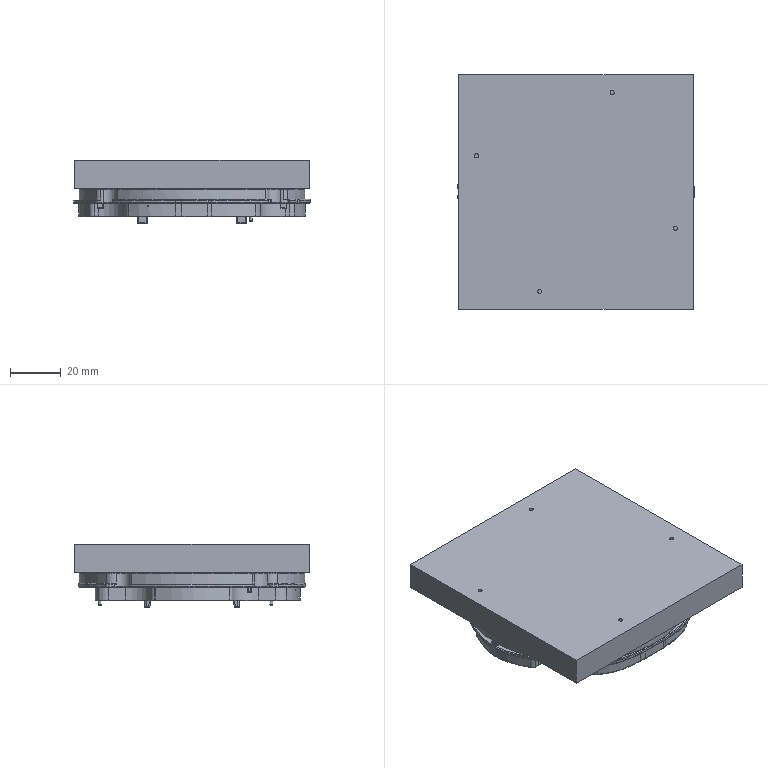NC program | NX | posted with a generic post | part box 92.935 x 92.1 x 24.829 mm
Lines 1 to 800 of 7643:
N10 G17 G21 G94 G90
(动态粗 , TOOL : D8-25-D8-60-3T-ROUGH)
N12 T10 M6
N14 G53
N16 G17 G0 G90 X-61.58 Y-2.72 S6500 M3
N18 G43 Z21. H10
N20 Z-16.5
N22 G94 G1 X-61.555 Y-2.718 Z-16.656 F3000.
N24 X-61.53 Y-2.716 Z-16.718
N26 X-61.505 Y-2.714 Z-16.763
N28 X-61.48 Y-2.712 Z-16.8
N30 X-61.455 Y-2.71 Z-16.831
N32 X-61.431 Y-2.708 Z-16.857
N34 X-61.406 Y-2.706 Z-16.88
N36 X-61.381 Y-2.704 Z-16.9
N38 X-61.356 Y-2.702 Z-16.918
N40 X-61.331 Y-2.7 Z-16.933
N42 X-61.306 Y-2.698 Z-16.947
N44 X-61.281 Y-2.696 Z-16.958
N46 X-61.256 Y-2.695 Z-16.968
N48 X-61.231 Y-2.693 Z-16.977
N50 X-61.206 Y-2.691 Z-16.984
N52 X-61.181 Y-2.689 Z-16.99
N54 X-61.156 Y-2.687 Z-16.994
N56 X-61.131 Y-2.685 Z-16.997
N58 X-61.107 Y-2.683 Z-16.999
N60 X-61.082 Y-2.681 Z-17.
N62 X-59.705 Y-2.575
N64 G3 X-59.048 Y-2.136 R0.809
N66 X-58.304 Y0.589 R7.458
N68 X-58.019 Y7.275 R66.093
N70 G1 X-57.999 Y15.352
N72 X-57.998 Y47.527
N74 G2 X-56.531 Y50.466 R4.191
N76 X-52.801 Y52.296 R8.355
N78 X-47.293 Y52.907 R28.085
N80 X-35.218 Y52.998 R429.952
N82 G1 X52.502
N84 G2 X55.445 Y51.539 R4.188
N86 X57.288 Y47.811 R8.352
N88 X57.906 Y42.305 R27.817
N90 X57.998 Y29.781 R440.504
N92 G1 X57.997 Y-47.524
N94 G2 X56.474 Y-50.512 R4.207
N96 X52.725 Y-52.312 R8.521
N98 X47.292 Y-52.907 R28.494
N100 X34.767 Y-52.998 R444.554
N102 G1 X-52.574 Y-52.996
N104 G2 X-55.546 Y-51.436 R4.252
N106 X-57.309 Y-47.741 R8.541
N108 X-57.906 Y-42.308 R28.316
N110 X-57.998 Y-29.784 R440.931
N112 G1 Y-5.349
N114 G2 X-57.574 Y-1.423 R34.883
N116 G3 X-57.04 Y7.367 R73.929
N118 X-56.999 Y17.527 R708.895
N120 G1 X-56.998 Y44.852
N122 G2 X-54.606 Y49.404 R5.85
N124 X-50.234 Y51.294 R10.717
N126 X-44.198 Y51.905 R34.632
N128 X-31.824 Y51.998 R454.909
N130 G1 X49.951 Y51.994
N132 G2 X54.419 Y49.578 R5.878
N134 X56.299 Y45.194 R10.811
N136 X56.913 Y38.933 R36.036
N138 X56.998 Y26.408 R512.708
N140 G1 X56.994 Y-44.973
N142 G2 X54.556 Y-49.44 R5.866
N144 X50.082 Y-51.323 R10.949
N146 X43.742 Y-51.919 R37.298
N148 X31.743 Y-51.998 R529.05
N150 G1 X-49.973 Y-51.994
N152 G2 X-54.479 Y-49.505 R5.891
N154 X-56.333 Y-45.038 R11.051
N156 X-56.92 Y-38.698 R37.895
N158 X-56.998 Y-26.249 R562.106
N160 G1 X-56.997 Y-7.449
N162 G2 X-56.543 Y-1.375 R62.284
N164 G3 X-56.019 Y10.497 R124.747
N166 G1 X-55.999 Y19.027
N168 X-55.998 Y42.527
N170 G2 X-52.754 Y48.527 R6.958
N172 X-47.94 Y50.343 R12.879
N174 X-41.372 Y50.916 R42.732
N176 X-28.622 Y50.997 R571.229
N178 G1 X47.528 Y50.996
N180 G2 X53.526 Y47.746 R6.968
N182 X55.341 Y42.934 R12.909
N184 X55.916 Y36.365 R42.803
N186 X55.997 Y23.541 R570.967
N188 G1 X55.996 Y-42.574
N190 G2 X52.819 Y-48.478 R6.937
N192 X48.018 Y-50.325 R12.706
N194 X41.302 Y-50.918 R42.332
N196 X28.552 Y-50.997 R585.104
N198 G1 X-47.523 Y-50.996
N200 G2 X-53.523 Y-47.754 R6.958
N202 X-55.326 Y-43.012 R12.809
N204 X-55.916 Y-36.371 R42.21
N206 X-55.997 Y-23.621 R569.284
N208 G1 X-55.996 Y-9.174
N210 G2 X-55.529 Y-1.349 R89.159
N212 G3 X-55.015 Y12.216 R166.099
N214 G1 X-54.999 Y20.452
N216 X-54.998 Y40.427
N218 G2 X-53.974 Y44.752 R8.324
N220 X-49.835 Y48.261 R8.776
N222 X-44.314 Y49.606 R18.927
N224 X-36.001 Y49.973 R85.068
N226 G1 X-26.101 Y49.997
N228 X45.377 Y49.996
N230 G2 X49.51 Y49.104 R8.517
N232 X53.139 Y45.091 R8.55
N234 X54.543 Y39.822 R17.669
N236 X54.966 Y31.662 R73.619
N238 G1 X54.997 Y20.937
N240 X54.996 Y-40.399
N242 G2 X54.094 Y-44.529 R8.451
N244 X50.067 Y-48.151 R8.576
N246 X44.642 Y-49.565 R18.027
N248 X36.556 Y-49.967 R76.51
N250 G1 X26.656 Y-49.997
N252 X-45.548 Y-49.995
N254 G2 X-50.109 Y-48.749 R8.039
N256 X-53.411 Y-44.473 R9.125
N258 X-54.661 Y-38.774 R20.599
N260 X-54.98 Y-30.083 R101.178
N262 G1 X-54.997 Y-21.008
N264 G2 X-54.956 Y-8.234 R650.637
N266 X-54.414 Y0.174 R225.645
N268 G3 X-54.007 Y14.834 R226.099
N270 G1 X-54. Y21.427
N272 X-53.997 Y38.627
N274 G2 X-53.323 Y42.594 R10.093
N276 X-49.146 Y46.885 R8.682
N278 X-43.617 Y48.48 R17.419
N280 X-36.061 Y48.945 R65.003
N282 X-24.361 Y48.997 R751.259
N284 G1 X43.614 Y48.994
N286 G2 X47.58 Y48.325 R10.167
N288 X51.868 Y44.173 R8.67
N290 X53.473 Y38.649 R17.352
N292 X53.946 Y31.018 R64.814
N294 X53.997 Y19.319 R752.456
N296 G1 X53.994 Y-38.681
N298 G2 X53.24 Y-42.78 R9.886
N300 X49.186 Y-46.86 R8.709
N302 X43.664 Y-48.47 R17.315
N304 X35.884 Y-48.948 R65.303
N306 X24.184 Y-48.996 R757.357
N308 G1 X-43.523 Y-48.995
N310 G2 X-47.427 Y-48.388 R10.486
N312 X-51.769 Y-44.358 R8.53
N314 X-53.431 Y-38.933 R16.692
N316 X-53.933 Y-31.68 R58.512
N318 X-53.997 Y-19.081 R756.083
N320 X-53.923 Y-8.124 R348.839
N322 X-53.366 Y1.045 R448.52
N324 G3 X-53.003 Y17.381 R286.219
N326 G1 X-53. Y22.327
N328 X-52.999 Y36.677
N330 G2 X-52.532 Y40.608 R13.005
N332 X-48.298 Y45.603 R8.772
N334 X-42.818 Y47.366 R16.685
N336 X-35.044 Y47.93 R57.999
N338 X-22.444 Y47.996 R751.574
N340 G1 X-12.214 Y47.997
N342 G2 X-2.428 Y48.649 R93.802
N344 X-0.938 Y48.456 R7.257
N346 G3 X0.999 Y48.473 R60.276
N348 G2 X2.359 Y48.649 R5.135
N350 X11.245 Y48.119 R116.377
N352 G3 X21.679 Y47.999 R281.98
N354 G1 X24.977 Y47.997
N356 X41.477 Y47.996
N358 G2 X45.272 Y47.626 R14.458
N360 X50.496 Y43.48 R8.662
N362 X52.329 Y38.029 R16.152
N364 X52.92 Y30.484 R54.023
N366 X52.996 Y17.809 R675.282
N368 G1 X52.994 Y-36.891
N370 G2 X52.438 Y-40.883 R12.008
N372 X48.27 Y-45.616 R8.807
N374 X42.718 Y-47.379 R16.873
N376 X34.868 Y-47.934 R59.591
N378 X22.268 Y-47.996 R759.278
N380 G1 X11.814 Y-47.997
N382 G2 X6.557 Y-48.462 R68.987
N384 X-10.972 Y-48.123 R114.357
N386 G3 X-21.625 Y-47.998 R270.066
N388 G1 X-41.374 Y-47.997
N390 G2 X-45.173 Y-47.653 R15.159
N392 X-50.487 Y-43.493 R8.652
N394 X-52.312 Y-38.122 R16.047
N396 X-52.917 Y-30.578 R52.808
N398 X-52.948 Y-9.629 R728.599
N400 X-52.409 Y0.369 R300.852
N402 G3 X-52.005 Y17.457 R297.752
N404 G1 X-52. Y22.402
N406 X-51.999 Y35.027
N408 G2 X-51.588 Y39.044 R15.182
N410 X-47.354 Y44.395 R8.967
N412 X-41.769 Y46.297 R16.488
N414 X-34.375 Y46.906 R52.937
N416 X-17.925 Y46.998 R776.352
N418 X-12.17 Y48.002 R46.605
N420 G3 X-19.006 Y46.734 R48.996
N422 G2 X-23.71 Y46.426 R32.015
N424 G3 X-35.146 Y46.267 R516.607
N426 X-42.15 Y45.534 R42.041
N428 X-47.261 Y43.465 R13.846
N430 X-50.907 Y37.704 R8.969
N432 X-51.354 Y32.556 R29.389
N434 X-51.405 Y17.729 R914.653
N436 G2 X-52.153 Y-5.249 R315.184
N438 G3 X-52.395 Y-17.47 R206.34
N440 X-52.267 Y-31.719 R423.43
N442 X-51.514 Y-38.644 R39.439
N444 X-49.463 Y-43.521 R13.03
N446 X-43.997 Y-46.903 R8.667
N448 X-38.923 Y-47.349 R29.196
N450 X-23.92 Y-47.396 R890.368
N452 G1 X-15.907 Y-47.421
N454 G3 X-10.698 Y-48.139 R66.308
N456 G2 X-18.604 Y-46.831 R55.637
N458 G3 X-23.932 Y-46.448 R37.065
N460 X-36.103 Y-46.381 R886.258
N462 G2 X-41.867 Y-46.095 R47.99
N464 X-46.751 Y-44.096 R9.428
N466 X-49.889 Y-39.361 R10.658
N468 X-51.067 Y-33.337 R24.634
N470 X-51.383 Y-23.369 R126.177
N472 X-51.305 Y-9.195 R466.749
N474 X-50.728 Y2.216 R781.354
N476 G3 X-50.404 Y19.705 R374.655
N478 G2 X-50.331 Y32.553 R530.644
N480 X-49.769 Y37.234 R21.015
N482 X-45.07 Y43.019 R9.193
N484 X-39.436 Y44.766 R17.581
N486 X-31.437 Y45.33 R61.997
N488 G3 X-22.401 Y45.493 R402.225
N490 X-20.942 Y46.075 R16.661
N492 G1 X-18.817 Y46.771
N494 G3 X-22.604 Y45.385 R31.53
N496 G2 X-25.744 Y44.909 R12.566
N498 X-33.704 Y44.648 R705.529
N500 G3 X-40.552 Y43.867 R39.499
N502 X-45.441 Y41.815 R13.41
N504 X-49.026 Y36.416 R9.392
N506 X-49.709 Y30.919 R25.341
N508 X-49.805 Y19.228 R391.929
N510 G2 X-49.981 Y6.512 R401.107
N512 G3 X-50.653 Y2.177 R33.083
N514 X-50.496 Y0.234 R12.796
N516 G2 X-50.624 Y-1.166 R2.803
N518 G3 X-50.587 Y-3.297 R17.335
N520 G2 X-50.73 Y-10.379 R211.012
N522 G3 X-50.67 Y-29.577 R444.123
N524 X-49.948 Y-36.506 R41.556
N526 X-47.926 Y-41.483 R13.371
N528 X-42.653 Y-45.017 R9.165
N530 X-37.232 Y-45.703 R24.779
N532 X-26.132 Y-45.82 R451.215
N534 G2 X-21.001 Y-46.012 R68.76
N536 G3 X-18.265 Y-46.898 R36.594
N538 G2 X-22.199 Y-45.53 R32.077
N540 G3 X-26.297 Y-44.949 R17.657
N542 X-34.934 Y-44.754 R275.021
N544 G2 X-40.608 Y-44.276 R34.269
N546 X-45.752 Y-41.66 R9.566
N548 X-48.538 Y-36.66 R11.811
N550 X-49.553 Y-30.226 R29.792
N552 X-49.787 Y-19.431 R179.128
N554 X-49.663 Y-7.748 R423.819
N556 X-50.625 Y-2.452 R36.382
N558 G3 X-49.674 Y-7.67 R35.094
N560 G2 X-49.258 Y-10.429 R10.113
N562 X-49.186 Y-19.33 R248.98
N564 G3 X-48.937 Y-30.05 R166.308
N566 X-47.909 Y-36.252 R27.806
N568 X-45.177 Y-40.933 R10.845
N570 X-40.373 Y-43.438 R10.384
N572 X-34.722 Y-44.107 R28.796
N574 G2 X-26.66 Y-44.353 R469.078
N576 X-24.143 Y-44.617 R21.733
N578 G3 X-22.172 Y-45.54 R26.904
N580 G2 X-24.917 Y-44.222 R32.855
N582 G3 X-28.254 Y-43.482 R11.563
N584 X-34.731 Y-43.094 R154.343
N586 G2 X-39.912 Y-42.322 R23.628
N588 X-46.104 Y-36.962 R9.673
N590 X-47.68 Y-31.115 R19.509
N592 X-48.139 Y-23.332 R71.778
N594 G1 X-48.209 Y-13.121
N596 G3 X-48.278 Y-11.836 R6.569
N598 G2 X-49.537 Y-8.137 R29.55
N600 G3 X-48.106 Y-12.277 R32.915
N602 G2 X-47.677 Y-15.66 R14.569
N604 X-47.499 Y-24.693 R957.139
N606 G3 X-46.872 Y-32.009 R50.54
N608 X-45.014 Y-37.292 R15.254
N610 X-39.499 Y-41.513 R9.823
N612 X-34.118 Y-42.457 R23.428
N614 G2 X-28.22 Y-42.929 R133.266
N616 X-26.525 Y-43.254 R8.785
N618 G1 X-24.718 Y-44.324
N620 G2 X-27.186 Y-42.819 R39.878
N622 G3 X-30.36 Y-41.939 R10.56
N624 G2 X-35.597 Y-41.263 R757.768
N626 X-40.36 Y-39.746 R14.148
N628 X-44.671 Y-34.763 R10.229
N630 X-46.148 Y-28.662 R21.487
N632 X-46.551 Y-21.1 R83.994
N634 G3 X-46.743 Y-15.442 R96.671
N636 X-47.494 Y-13.733 R27.048
N638 G1 X-48.181 Y-12.07
N640 G3 X-46.588 Y-15.767 R116.697
N642 G2 X-46.097 Y-18.895 R13.324
N644 G1 X-45.77 Y-25.752
N646 G3 X-44.802 Y-32.193 R31.449
N648 X-42.14 Y-37.171 R11.835
N650 X-37.218 Y-40.071 R10.973
N652 X-32.11 Y-41.072 R35.641
N654 G2 X-28.701 Y-41.755 R24.025
N656 X-27.031 Y-42.909 R28.
N658 X-29.059 Y-41.419 R22.396
N660 G3 X-31.754 Y-40.376 R9.271
N662 G2 X-36.132 Y-39.251 R75.156
N664 X-41.436 Y-35.754 R10.775
N666 X-43.922 Y-30.413 R13.767
N668 X-44.802 Y-23.957 R36.812
N670 G3 X-45.17 Y-18.68 R98.427
N672 G1 X-46.659 Y-15.585
N674 X-45.008 Y-18.983
N676 G2 X-44.404 Y-22.156 R13.593
N678 G3 X-43.708 Y-28.164 R86.126
N680 X-41.923 Y-33.553 R16.796
N682 X-36.49 Y-38.227 R10.796
N684 X-32.271 Y-39.598 R38.921
N686 G2 X-30.454 Y-40.227 R18.329
N688 G1 X-28.905 Y-41.532
N690 G2 X-30.932 Y-39.761 R34.939
N692 G3 X-33.274 Y-38.517 R11.416
N694 G2 X-37.068 Y-36.655 R24.972
N696 X-41.678 Y-30.788 R11.687
N698 X-43.019 Y-24.95 R26.219
N700 G3 X-43.438 Y-21.958 R335.773
N702 G1 X-45.081 Y-18.815
N704 G3 X-43.216 Y-22.365 R447.582
N706 G2 X-42.491 Y-25.075 R16.311
N708 G3 X-41.179 Y-30.08 R31.83
N710 X-35.498 Y-36.627 R12.158
N712 G1 X-32.491 Y-38.207
N714 X-30.792 Y-39.881
N716 G2 X-33.112 Y-37.47 R32.523
N718 G3 X-35.722 Y-35.365 R61.614
N720 G2 X-40.398 Y-28.487 R14.563
N722 X-41.206 Y-25.828 R116.518
N724 X-43.311 Y-22.161 R75.506
N726 G3 X-41.37 Y-25.584 R346.156
N728 G2 X-40.263 Y-27.536 R8.47
N730 G3 X-38.083 Y-31.671 R24.809
N732 X-34.821 Y-35.177 R19.008
N734 G2 X-33.968 Y-36.464 R91.324
N736 G1 X-32.985 Y-37.597
N738 G2 X-34.619 Y-35.498 R13.241
N740 G3 X-35.821 Y-33.292 R10.755
N742 G2 X-38.875 Y-28.029 R48.011
N744 G1 X-39.03 Y-27.866
N746 G2 X-40.705 Y-26.489 R7.646
N748 G1 X-41.06 Y-26.006
N750 X-40.705 Y-26.489
N752 G3 X-38.908 Y-27.945 R7.826
N754 G2 X-37.422 Y-29.807 R9.645
N756 X-35.461 Y-32.799 R156.161
N758 X-35.374 Y-33.303 R1.645
N760 G1 X-35.092 Y-34.434
N762 X-35.001 Y-34.639
N764 G2 X-35.425 Y-32.577 R6.115
N766 G3 X-36.662 Y-29.587 R9.097
N768 X-37.361 Y-28.611 R4.628
N770 X-37.953 Y-28.378 R1.522
N772 G1 X-38.972 Y-27.906
N774 X-37.953 Y-28.378
N776 G2 X-36.723 Y-29.1 R1.909
N778 X-35.405 Y-31.301 R6.68
N780 X-35.456 Y-32.142 R3.094
N782 G1 X-35.424 Y-32.59
N784 G2 X-35.389 Y-31.498 R3.522
N786 G3 X-35.852 Y-29.445 R3.065
N788 X-36.491 Y-28.75 R1.511
N790 G1 X-37.52 Y-28.496
N792 G3 X-36.466 Y-28.72 R4.38
N794 G2 X-35.322 Y-30.038 R2.305
N796 X-35.335 Y-30.983 R1.189
N798 G1 X-35.351 Y-31.132
N800 G2 X-35.176 Y-30.423 R5.061
N802 G3 X-35.753 Y-28.876 R1.638
N804 X-36.601 Y-28.7 R1.92
N806 G1 X-35.855 Y-28.78
N808 G2 X-35.074 Y-30.064 R1.25
N810 G1 X-35.176 Y-30.425
N812 G3 X-34.996 Y-29.647 R4.512
N814 X-35.969 Y-28.762 R0.921
N816 X-36.593 Y-28.973 R0.803
N818 G1 X-36.943 Y-29.299
N820 X-38.087 Y-30.366 Z-16.9
N822 G2 X-39.018 Y-30.522 R0.803 F15000.
N824 G1 X-39.673 Y-30.194
N826 X-40.324 Y-29.857
N828 G2 X-41.806 Y-28.867 R10.095
N830 X-42.83 Y-27.639 R4.698
N832 G1 X-44.026 Y-25.565
N834 X-45.215 Y-23.487
N836 G2 X-48.507 Y-17.159 R115.865
N838 X-51.398 Y-10.117 R71.891
N840 X-52.234 Y-7.344 R44.136
N842 X-52.741 Y-4.7 R22.374
N844 G1 X-52.958 Y-3.027
N846 G2 X-52.614 Y-2.263 R0.801
N848 G1 X-51.326 Y-1.373 Z-17. F3000.
N850 X-51.009 Y-1.157
N852 X-50.7 Y-0.931
N854 G3 X-50.468 Y-0.538 R0.814
N856 X-50.406 Y0.31 R1.534
N858 G1 X-50.625 Y1.193
N860 X-50.653 Y2.177
N862 G2 X-50.368 Y4.504 R30.875
N864 X-49.365 Y8.916 R48.271
N866 G3 X-48.895 Y14.022 R31.072
N868 X-48.781 Y26.909 R644.328
N870 G2 X-48.431 Y33.495 R52.792
N872 X-46.843 Y38.145 R11.412
N874 X-42.08 Y41.953 R10.192
N876 X-36.108 Y43.358 R21.859
N878 X-28.168 Y43.808 R109.95
N880 G3 X-25.391 Y44.004 R39.396
N882 X-24.999 Y44.204 R2.842
N884 G2 X-22.591 Y45.391 R33.125
N886 G3 X-25.524 Y43.904 R31.271
N888 G2 X-28.22 Y43.344 R9.885
N890 X-34.501 Y42.886 R755.129
N892 G3 X-40.459 Y41.769 R26.181
N894 X-45.27 Y38.67 R10.587
N896 X-47.559 Y33.677 R11.137
N898 X-48.138 Y27.488 R34.991
N900 X-48.24 Y16.873 R884.24
N902 G2 X-48.491 Y11.33 R65.646
N904 G3 X-49.467 Y8.491 R54.281
N906 G2 X-47.957 Y12.688 R50.945
N908 G3 X-47.375 Y16.666 R18.146
N910 X-47.163 Y25.885 R238.666
N912 G2 X-46.689 Y32.161 R41.673
N914 X-44.698 Y37.045 R11.146
N916 X-39.813 Y40.522 R10.861
N918 X-33.968 Y41.807 R24.231
N920 G3 X-28.421 Y42.364 R323.329
N922 X-27.564 Y42.567 R2.429
N924 G2 X-25.307 Y44.017 R24.433
N926 G3 X-27.685 Y42.479 R24.542
N928 G2 X-29.804 Y41.798 R6.558
N930 X-34.852 Y41.067 R238.638
N932 G3 X-40.171 Y39.547 R19.422
N934 X-45.552 Y33.222 R10.006
N936 X-46.451 Y27.456 R24.19
N938 X-46.689 Y18.889 R416.558
N940 G2 X-46.998 Y14.897 R37.516
N942 G1 X-47.991 Y12.581
N944 G2 X-46.498 Y15.952 R93.021
N946 G3 X-45.825 Y19.661 R14.909
N948 X-45.49 Y26.341 R291.055
N950 G2 X-44.689 Y31.897 R25.594
N952 X-39.086 Y38.472 R10.119
N954 X-33.855 Y40.055 R21.227
N956 G3 X-29.864 Y40.835 R75.673
N958 G1 X-29.606 Y40.969
N960 G2 X-27.626 Y42.522 R15.785
N962 G3 X-29.778 Y40.824 R17.362
N964 G2 X-31.96 Y39.966 R7.743
N966 G3 X-36.392 Y38.779 R77.204
N968 X-41.178 Y36.055 R12.3
N970 X-44.108 Y30.793 R11.117
N972 X-44.917 Y24.857 R30.653
N974 G2 X-45.366 Y18.74 R90.011
N976 X-45.501 Y18. R11.468
N978 G1 X-46.572 Y15.769
N980 X-44.934 Y19.18
N982 G3 X-44.207 Y22.628 R15.053
N984 G2 X-43.549 Y28.083 R105.738
N986 X-41.816 Y33.004 R13.614
N988 X-37.02 Y37.085 R11.045
N990 X-32.508 Y38.726 R38.5
N992 G3 X-31.619 Y39.096 R3.163
N994 G2 X-29.704 Y40.884 R21.086
N996 G3 X-31.778 Y38.937 R22.587
N998 G2 X-33.872 Y37.809 R9.504
N1000 G3 X-37.796 Y35.844 R25.277
N1002 X-42.323 Y29.717 R11.079
N1004 X-43.373 Y24.351 R30.532
N1006 G2 X-43.904 Y21.082 R27.325
N1008 G1 X-45.058 Y18.892
N1010 G3 X-43.242 Y22.363 R539.919
N1012 X-42.419 Y25.165 R18.609
N1014 G2 X-41.093 Y29.701 R27.337
N1016 X-36.311 Y35.175 R11.78
N1018 G1 X-33.935 Y36.559
N1020 X-32.277 Y38.443
N1022 X-31.744 Y38.971
N1024 G3 X-34.095 Y36.343 R34.059
N1026 G2 X-36.293 Y34.52 R25.762
N1028 G3 X-40.945 Y27.825 R13.716
N1030 X-41.891 Y24.704 R159.879
N1032 G1 X-43.368 Y22.093
N1034 X-41.529 Y25.345
N1036 G3 X-39.904 Y28.126 R21.532
N1038 G2 X-35.848 Y33.326 R18.403
N1040 G3 X-35.236 Y33.977 R2.888
N1042 G2 X-33.958 Y36.501 R6.809
N1044 G1 X-34.563 Y35.643
N1046 X-35.066 Y34.563
N1048 G2 X-35.8 Y32.973 R3.417
N1050 G3 X-38.567 Y29.079 R49.359
N1052 G2 X-39.474 Y27.602 R18.195
N1054 G3 X-40.952 Y26.202 R6.694
N1056 G2 X-40.053 Y27.17 R9.352
N1058 G3 X-37.072 Y29.899 R12.939
N1060 X-35.547 Y31.843 R19.81
N1062 X-35.464 Y32.223 R1.563
N1064 G1 X-35.369 Y33.411
N1066 X-35.216 Y33.991
N1068 X-35.369 Y33.411
N1070 G2 X-35.479 Y31.878 R66.65
N1072 X-36.736 Y29.643 R7.055
N1074 X-37.736 Y28.506 R8.458
N1076 G1 X-39.104 Y27.858
N1078 G2 X-37.936 Y28.402 R10.366
N1080 G3 X-36.344 Y29.366 R3.278
N1082 X-35.374 Y30.689 R4.121
N1084 X-35.352 Y31.088 R1.583
N1086 G1 X-35.455 Y32.133
N1088 G3 X-35.312 Y30.892 R13.973
N1090 G2 X-35.946 Y29.418 R2.524
N1092 X-36.762 Y28.721 R1.919
N1094 G1 X-37.642 Y28.486
N1096 G2 X-36.479 Y28.758 R7.377
N1098 G3 X-35.165 Y30.055 R2.067
N1100 G1 X-35.167 Y30.404
N1102 X-35.331 Y30.981
N1104 G2 X-35.117 Y30.072 R3.557
N1106 X-36.057 Y28.798 R1.629
N1108 G1 X-36.702 Y28.713
N1110 G3 X-35.671 Y28.883 R3.444
N1112 X-35.04 Y29.956 R1.011
N1114 G1 X-35.143 Y30.317
N1116 G2 X-35.037 Y29.443 R1.549
N1118 X-35.97 Y28.787 R0.934
N1120 G3 X-35.468 Y28.906 R1.316
N1122 X-35.014 Y29.56 R0.871
N1124 X-35.77 Y30.446 R0.8
N1126 G1 X-35.917 Y30.453
N1128 X-37.39 Y30.53 Z-16.906
N1130 X-37.477 Y30.549 Z-16.9
N1132 G2 X-38.063 Y31.32 R0.8 F15000.
N1134 X-38.016 Y32.456 R7.552
N1136 G1 X-37.796 Y33.524
N1138 X-37.55 Y34.587
N1140 G2 X-36.48 Y37.083 R8.875
N1142 G1 X-36.26 Y37.404
N1144 X-36.028 Y37.716
N1146 X-35.319 Y38.608
N1148 X-34.584 Y39.478
N1150 G2 X-32.755 Y41.327 R24.194
N1152 G1 X-31.593 Y42.384
N1154 X-30.419 Y43.428
N1156 G2 X-26.577 Y46.05 R22.943
N1158 X-18.898 Y49.106 R30.417
N1160 X-13.631 Y50.128 R43.509
N1162 X-6.824 Y50.765 R76.806
N1164 X0.99 Y51.054 R184.717
N1166 G1 X9.217 Y51.181
N1168 G2 X10.021 Y50.498 R0.8
N1170 G1 X10.062 Y50.218
N1172 X10.284 Y48.741 Z-16.995 F3000.
N1174 X10.303 Y48.673 Z-17.
N1176 G3 X10.977 Y48.133 R0.801
N1178 G2 X16.545 Y47.332 R76.355
N1180 G3 X22.465 Y47.031 R55.096
N1182 X31.727 Y46.997 R689.581
N1184 G2 X41.427 Y46.965 R450.818
N1186 X46.283 Y45.611 R9.748
N1188 X50.063 Y41.047 R9.997
N1190 X51.547 Y35.022 R20.976
N1192 X51.961 Y26.485 R86.19
N1194 G1 X51.996 Y15.235
N1196 X51.995 Y-35.04
N1198 G2 X51.583 Y-39.056 R15.145
N1200 X47.307 Y-44.419 R8.975
N1202 X41.79 Y-46.29 R16.504
N1204 X34.397 Y-46.904 R52.63
N1206 X17.826 Y-46.997 R749.451
N1208 X13.677 Y-47.784 R53.562
N1210 G1 X11.74 Y-48.005
N1212 G3 X18.684 Y-46.764 R41.986
N1214 G2 X23.101 Y-46.435 R27.603
N1216 G3 X34.524 Y-46.289 R840.828
N1218 X41.76 Y-45.611 R46.53
N1220 X46.929 Y-43.685 R14.712
N1222 X50.891 Y-37.764 R8.937
N1224 X51.35 Y-32.541 R29.249
N1226 X51.396 Y-23.541 R654.83
N1228 G1 X51.394 Y19.084
N1230 G3 X51.21 Y31.381 R260.532
N1232 X50.298 Y38.133 R33.717
N1234 X47.858 Y43.03 R12.054
N1236 X42.557 Y45.933 R9.111
N1238 X37.33 Y46.356 R31.525
N1240 X24.823 Y46.411 R912.851
N1242 G2 X19.406 Y46.547 R89.898
N1244 G1 X18.32 Y46.888
N1246 X16.076 Y47.402
N1248 G2 X20.903 Y46.065 R34.62
N1250 G3 X24.887 Y45.536 R18.824
N1252 X34.666 Y45.384 R245.978
N1254 G2 X40.58 Y45.095 R49.107
N1256 X45.535 Y43.109 R9.801
N1258 X48.803 Y38.311 R10.818
N1260 X50.038 Y32.228 R24.379
N1262 X50.377 Y22.712 R115.634
N1264 G1 X50.395 Y13.787
N1266 X50.398 Y3.595
N1268 X50.527 Y2.671
N1270 X50.667 Y0.008
N1272 G3 X50.398 Y-12.052 R188.955
N1274 G1 X50.396 Y-15.949
N1276 G2 X50.34 Y-32.099 R889.013
N1278 X49.839 Y-36.939 R23.898
N1280 X45.005 Y-43.049 R9.2
N1282 X39.434 Y-44.764 R17.687
N1284 X31.36 Y-45.331 R62.152
N1286 G3 X22.369 Y-45.482 R534.038
N1288 G1 X22.191 Y-45.516
N1290 G2 X18.297 Y-46.856 R34.126
N1292 G3 X22.571 Y-45.357 R34.242
N1294 G2 X25.713 Y-44.903 R13.405
N1296 X33.53 Y-44.654 R727.78
N1298 G3 X40.381 Y-43.903 R40.99
N1300 X45.35 Y-41.875 R13.718
N1302 X49.012 Y-36.451 R9.37
N1304 X49.704 Y-30.956 R25.081
N1306 X49.795 Y-21.057 R314.677
N1308 G2 X49.838 Y-6.744 R890.09
N1310 G1 X50.227 Y-4.923
N1312 X50.547 Y-2.466
N1314 G2 X49.709 Y-7.346 R35.696
N1316 G3 X48.969 Y-11.429 R14.208
N1318 X48.797 Y-21.128 R170.748
N1320 G2 X48.666 Y-30.951 R213.869
N1322 X47.889 Y-35.902 R19.816
N1324 X43.007 Y-41.517 R9.479
N1326 X37.337 Y-43.195 R18.326
N1328 X30.161 Y-43.732 R65.261
N1330 G3 X25.297 Y-44.005 R55.118
N1332 X23.846 Y-44.753 R28.064
N1334 G1 X22.348 Y-45.444
N1336 G3 X25.437 Y-43.902 R32.748
N1338 G2 X28.191 Y-43.338 R10.206
N1340 X34.327 Y-42.9 R744.095
N1342 G3 X40.364 Y-41.797 R26.811
N1344 X45.091 Y-38.87 R10.749
N1346 X47.516 Y-33.857 R10.876
N1348 X48.124 Y-27.821 R32.708
N1350 X48.228 Y-16.042 R907.607
N1352 G2 X48.441 Y-11.208 R52.665
N1354 G3 X49.363 Y-8.497 R24.862
N1356 G2 X48. Y-12.37 R40.328
N1358 G3 X47.386 Y-16.09 R15.046
N1360 X47.182 Y-24.303 R149.178
N1362 G2 X46.834 Y-31.191 R61.029
N1364 X45.397 Y-35.974 R13.238
N1366 X40.681 Y-40.156 R10.046
N1368 X34.828 Y-41.697 R20.666
N1370 X29.011 Y-42.282 R255.233
N1372 G3 X27.573 Y-42.513 R8.729
N1374 G2 X25.23 Y-44.009 R100.162
N1376 G3 X27.624 Y-42.451 R29.488
N1378 G2 X29.955 Y-41.756 R7.554
N1380 X35.069 Y-41.028 R922.199
N1382 G3 X40.367 Y-39.448 R18.653
N1384 X45.524 Y-33.3 R9.956
N1386 X46.436 Y-27.613 R23.572
N1388 X46.663 Y-19.092 R296.707
N1390 G2 X46.968 Y-14.803 R41.413
N1392 G1 X48.007 Y-12.353
N1394 G2 X46.469 Y-15.872 R208.966
N1396 G3 X45.81 Y-19.575 R15.007
N1398 X45.469 Y-26.556 R340.403
N1400 G2 X44.667 Y-31.96 R24.761
N1402 X39.064 Y-38.479 R10.12
N1404 X33.83 Y-40.055 R21.205
N1406 G3 X29.744 Y-40.849 R69.915
N1408 X28.961 Y-41.457 R3.321
N1410 G1 X27.515 Y-42.529
N1412 G3 X29.637 Y-40.868 R23.092
N1414 G2 X31.734 Y-40.014 R6.812
N1416 G3 X36.221 Y-38.83 R101.767
N1418 X41.047 Y-36.177 R12.598
N1420 X44.071 Y-30.913 R10.971
N1422 X44.891 Y-25.131 R28.968
N1424 G2 X45.312 Y-18.924 R119.468
N1426 X45.486 Y-17.88 R10.266
N1428 G1 X46.547 Y-15.679
N1430 X44.961 Y-18.946
N1432 G3 X44.221 Y-22.331 R13.946
N1434 G2 X43.581 Y-27.851 R130.729
N1436 X41.969 Y-32.743 R14.186
N1438 X37.151 Y-37.013 R10.855
N1440 X32.769 Y-38.623 R32.682
N1442 G3 X31.583 Y-39.065 R6.455
N1444 G2 X29.602 Y-40.9 R22.571
N1446 G3 X31.62 Y-39.01 R19.034
N1448 G2 X33.481 Y-37.959 R7.382
N1450 G3 X37.295 Y-36.147 R34.701
N1452 X42.295 Y-29.785 R11.03
N1454 X43.29 Y-24.865 R27.557
N1456 G2 X43.872 Y-21.016 R45.24
N1458 G1 X45.035 Y-18.779
N1460 X43.246 Y-22.213
N1462 G3 X42.418 Y-25.069 R18.459
N1464 G2 X41.149 Y-29.544 R28.172
N1466 X36.293 Y-35.17 R11.725
N1468 X33.802 Y-36.605 R137.573
N1470 X31.591 Y-39.04 R36.441
N1472 G3 X34.008 Y-36.352 R36.154
N1474 G2 X36.302 Y-34.484 R30.369
N1476 G3 X40.924 Y-27.842 R13.542
N1478 X41.907 Y-24.552 R124.215
N1480 G1 X43.375 Y-21.936
N1482 X41.373 Y-25.474
N1484 G3 X40.06 Y-27.775 R16.759
N1486 G2 X35.57 Y-33.544 R18.669
N1488 G3 X35.021 Y-34.446 R1.28
N1490 G2 X33.892 Y-36.478 R7.839
N1492 G3 X35.021 Y-34.446 R7.837
N1494 G2 X35.691 Y-33.05 R3.018
N1496 G3 X38.32 Y-29.427 R52.041
N1498 G2 X39.452 Y-27.558 R85.542
N1500 G1 X39.899 Y-27.218
N1502 X40.711 Y-26.41
N1504 X41.144 Y-25.798
N1506 G2 X39.55 Y-27.464 R5.915
N1508 G3 X37.497 Y-29.346 R9.441
N1510 X35.483 Y-31.837 R27.452
N1512 X35.385 Y-32.211 R1.62
N1514 G1 X35.306 Y-33.314
N1516 X35.123 Y-34.042
N1518 X35.306 Y-33.314
N1520 X35.387 Y-32.
N1522 G2 X36.344 Y-30.096 R5.502
N1524 X37.684 Y-28.481 R9.447
N1526 G1 X38.962 Y-27.877
N1528 G2 X37.463 Y-28.51 R8.157
N1530 G3 X35.313 Y-30.661 R4.925
N1532 G1 X35.269 Y-30.99
N1534 X35.389 Y-32.15
N1536 X35.243 Y-30.842
N1538 G2 X36.066 Y-29.188 R2.901
N1540 X36.822 Y-28.672 R1.351
N1542 G1 X37.617 Y-28.452
N1544 G2 X36.436 Y-28.729 R7.124
N1546 G3 X35.111 Y-29.989 R2.222
N1548 X35.099 Y-30.391 R1.723
N1550 G1 X35.269 Y-30.99
N1552 G2 X35.048 Y-30.066 R3.708
N1554 X35.985 Y-28.778 R1.662
N1556 X36.577 Y-28.696 R9.956
N1558 G3 X35.626 Y-28.852 R3.145
N1560 X34.972 Y-29.946 R1.028
N1562 G1 X35.095 Y-30.379
N1564 G2 X34.946 Y-29.499 R2.017
N1566 X35.75 Y-28.779 R0.883
N1568 G1 X35.974 Y-28.756
N1570 G3 X35.396 Y-28.882 R1.564
N1572 X34.942 Y-29.536 R0.87
N1574 X35.354 Y-30.325 R0.801
N1576 G1 X35.889 Y-30.617
N1578 X37.265 Y-31.361 Z-16.9
N1580 G3 X37.991 Y-31.296 R0.802 F15000.
N1582 G1 X39.399 Y-30.412
N1584 X40.799 Y-29.514
N1586 G3 X43.163 Y-26.986 R8.214
N1588 X46.981 Y-20.16 R106.117
N1590 X50.27 Y-13.073 R86.749
N1592 X52.373 Y-6.471 R47.348
N1594 X52.763 Y-4.161 R22.303
N1596 G1 X53.446 Y1.835
N1598 G3 X52.744 Y2.72 R0.8